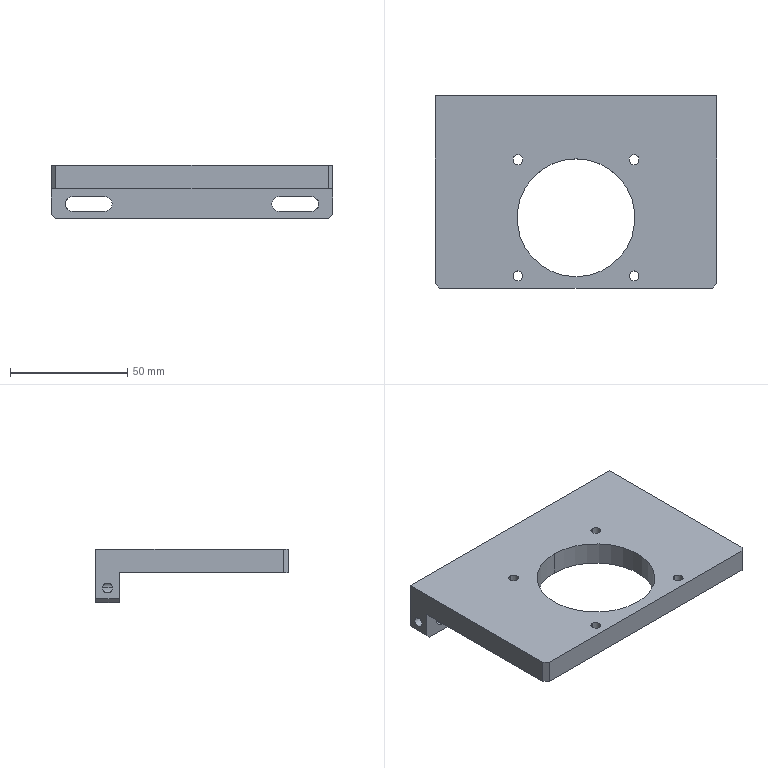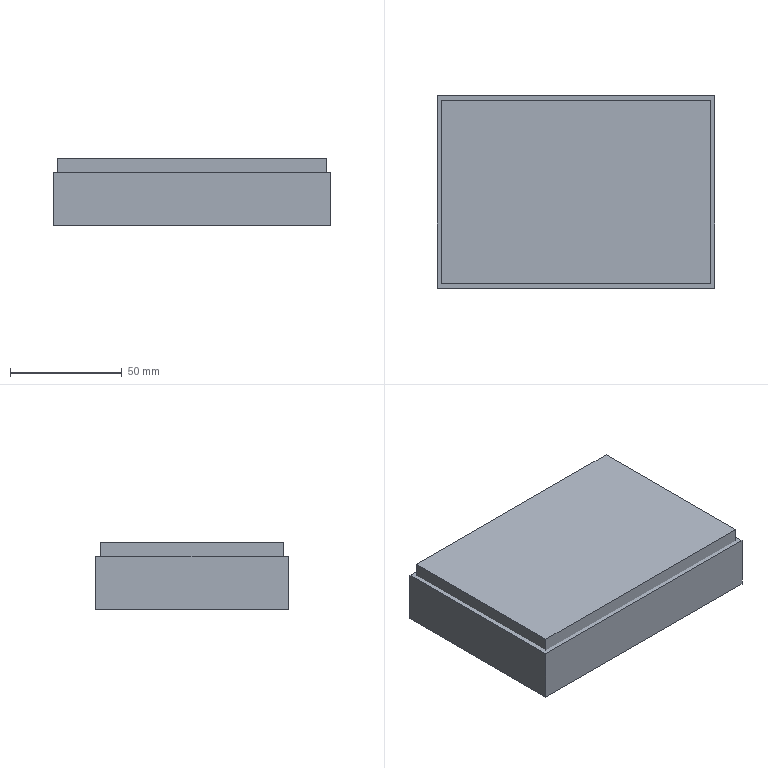CAM job | NX | 3+2 milling, drilling | part box 120 x 82 x 22.8 mm | stock box 124 x 86 x 29.8 mm
Tools:
number,name,description,diameter,corner_radius,flute_length,length,flutes
19,D80,Milling Tool-5 Parameters,80.0,0.0,50.0,75.0,2
15,D10,Milling Tool-5 Parameters,10.0,0.0,50.0,75.0,2
14,D10JING,Milling Tool-5 Parameters,10.0,0.0,50.0,75.0,2
1,D6A45,Milling Tool-5 Parameters,6.0,0.0,50.0,75.0,2
4,4.2ZT,Drilling Tool,4.2,0.0,35.0,50.0,2
11,D4,Milling Tool-5 Parameters,4.0,0.0,50.0,75.0,2
Operations:
program,operation,operation_type,tool,method,geometry_group,spindle_rpm,surface_speed,feed_per_tooth,feed_cut,feed_plunge,cut_length_mm,path_length_mm,cut_time_min,machine_time_min
1,FLOOR_WALL,VolumeBased25DMillingOperation,D80,METHOD,A,6500.0,1633.0,0.1154,1500.0,100.0,677.997,731.997,0.452,0.4574
1,ZLEVEL_PROFILE,ZLevelMilling,D10,METHOD,A,9500.0,298.0,0.1579,3000.0,1000.0,10457.67,10537.47,3.518,3.526
1,ZLEVEL_PROFILE_COPY,ZLevelMilling,D10,METHOD,A,9500.0,298.0,0.1579,3000.0,1000.0,1430.55,1497.55,0.5087,0.5154
1,ZLEVEL_PROFILE_1,ZLevelMilling,D10JING,METHOD,A,9500.0,298.0,0.0789,1500.0,1000.0,1307.694,1398.894,0.8731,0.8823
1,ZLEVEL_PROFILE_1_COPY,ZLevelMilling,D10JING,METHOD,A,9500.0,298.0,0.0789,1500.0,1000.0,347.526,414.526,0.3049,0.3116
1,DRILLING,Operation,D6A45,METHOD,A,9500.0,179.0,0.0132,250.0,0.0,16.0,270.241,0.064,0.0894
1,DRILLING_COPY_COPY,Operation,4.2ZT,METHOD,A,2000.0,21.0,0.0375,150.0,0.0,63.047,343.859,0.4203,0.4484
1,PLANAR_MILL,PlanarMilling,D6A45,METHOD,A,9500.0,179.0,0.0658,1250.0,100.0,620.091,1181.221,0.4961,0.5522
2,FLOOR_WALL_COPY,VolumeBased25DMillingOperation,D80,METHOD,B,6500.0,1633.0,0.1154,1500.0,100.0,4633.979,6241.863,3.089,3.25
2,FLOOR_WALL_1,VolumeBased25DMillingOperation,D10,METHOD,B,9500.0,298.0,0.1579,3000.0,100.0,19031.733,19569.566,6.344,6.398
2,FLOOR_WALL_1_COPY,VolumeBased25DMillingOperation,D10JING,METHOD,B,9500.0,298.0,0.0789,1500.0,100.0,2159.088,2375.689,1.439,1.461
2,PLANAR_MILL_COPY,PlanarMilling,D6A45,METHOD,B,9500.0,179.0,0.0658,1250.0,100.0,270.749,329.749,0.2166,0.2225
2,PLANAR_MILL_COPY_COPY_1,PlanarMilling,D6A45,METHOD,B,9500.0,179.0,0.0658,1250.0,100.0,69.153,467.612,0.0553,0.0952
2,PLANAR_MILL_COPY_COPY,PlanarMilling,D6A45,METHOD,B,9500.0,179.0,0.0658,1250.0,100.0,486.063,1203.027,0.3889,0.4605
3,ZLEVEL_PROFILE_COPY_1,ZLevelMilling,D4,METHOD,C,9500.0,119.0,0.0789,1500.0,1000.0,1869.065,2142.98,1.27,1.298
3,PLANAR_MILL_COPY_COPY_2,PlanarMilling,D6A45,METHOD,C,9500.0,179.0,0.0658,1250.0,100.0,387.504,657.728,0.31,0.337